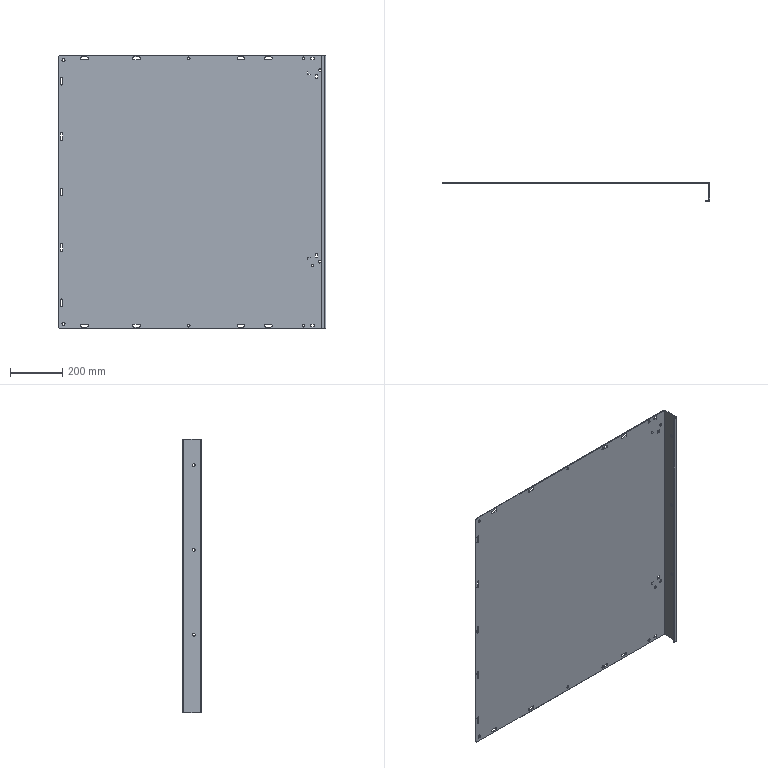Part | 1 solid | 133 faces | box 1025 x 70 x 1050 mm | volume 3456930 mm3 | plane 68 | cylinder 65 | commonest cylinder face diameters 10 x43 10.5 x12 12 x4 0.4 x2 6.4 x2 24 x2